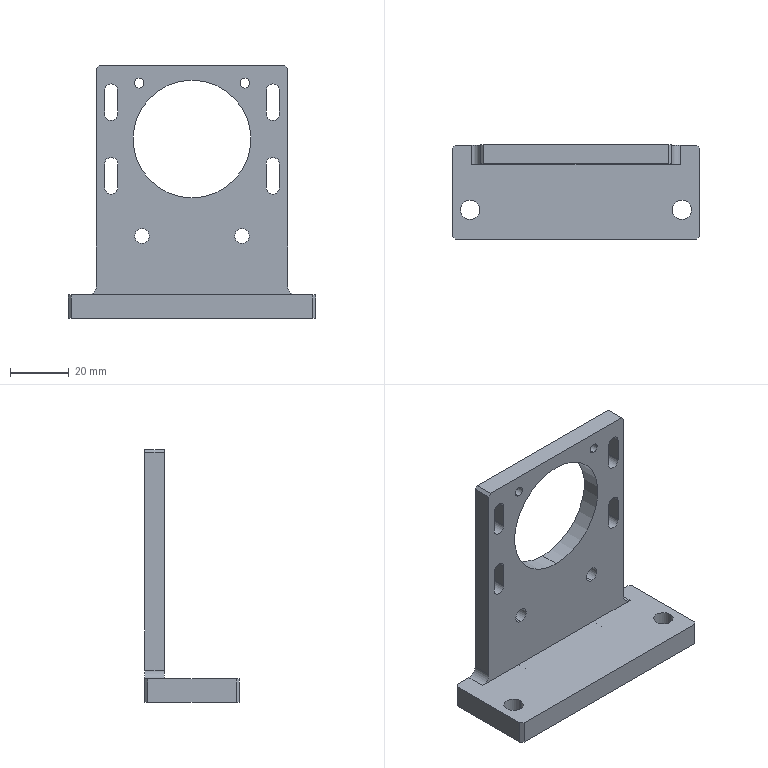Part | STEP file | Motor adapter plate | 1 solid | 60 faces | box 84 x 32 x 86 mm | volume 43828 mm3 | cylinder 32 | plane 24 | cone 4 | commonest cylinder face diameters 4.5 x12 3.3 x8 5 x4 6.6 x4 6 x2 40 x2